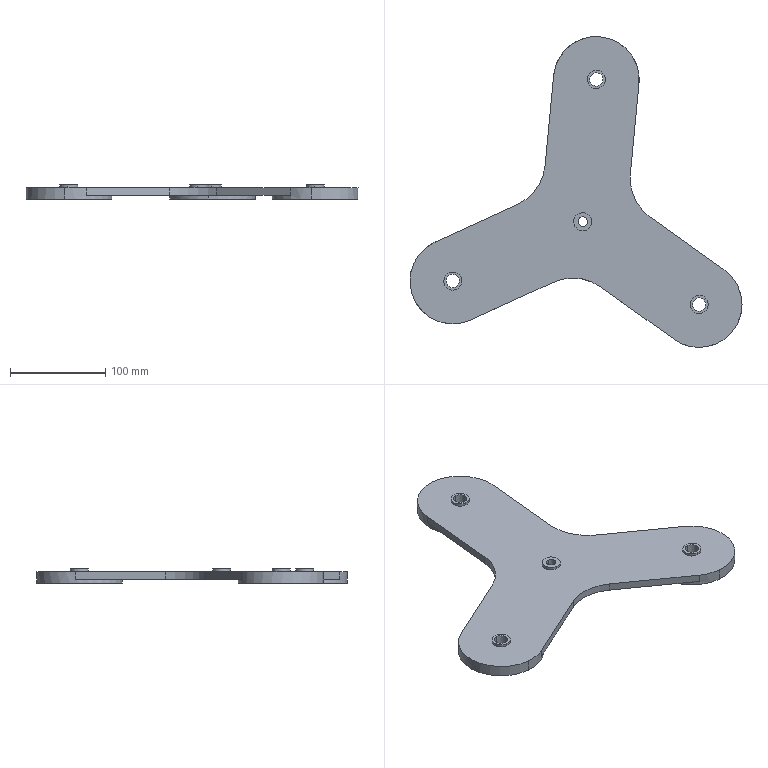Part | SolidWorks | features BaseBody 1 | 1 solid | 40 faces | box 348.636 x 326.309 x 15 mm | volume 447458 mm3 | cylinder 25 | plane 15 | commonest cylinder face diameters 19 x8 14 x6 90 x6 100 x3 10 x2
STEP:
#1=CARTESIAN_POINT('',(358.485,52.161,-468.));
#2=VERTEX_POINT('',#1);
#3=CARTESIAN_POINT('',(359.433,62.116,-468.));
#4=VERTEX_POINT('',#3);
#5=CARTESIAN_POINT('',(358.959,57.138,-468.));
#6=DIRECTION('',(0.,0.,-1.));
#7=DIRECTION('',(0.09487,0.9955,0.));
#8=AXIS2_PLACEMENT_3D('',#5,#6,#7);
#9=CIRCLE('',#8,5.);
#10=EDGE_CURVE('',#2,#4,#9,.T.);
#11=ORIENTED_EDGE('',*,*,#10,.T.);
#12=CARTESIAN_POINT('',(359.433,62.116,-457.));
#13=VERTEX_POINT('',#12);
#14=CARTESIAN_POINT('',(359.433,62.116,-472.));
#15=DIRECTION('',(0.,0.,1.));
#16=VECTOR('',#15,1000.);
#17=LINE('',#14,#16);
#18=EDGE_CURVE('',#4,#13,#17,.T.);
#19=ORIENTED_EDGE('',*,*,#18,.T.);
#20=CARTESIAN_POINT('',(358.485,52.161,-457.));
#21=VERTEX_POINT('',#20);
#22=CARTESIAN_POINT('',(358.959,57.138,-457.));
#23=DIRECTION('',(0.,0.,1.));
#24=DIRECTION('',(-0.09487,-0.9955,0.));
#25=AXIS2_PLACEMENT_3D('',#22,#23,#24);
#26=CIRCLE('',#25,5.);
#27=EDGE_CURVE('',#13,#21,#26,.T.);
#28=ORIENTED_EDGE('',*,*,#27,.T.);
#29=CARTESIAN_POINT('',(358.485,52.161,-472.));
#30=DIRECTION('',(0.,0.,1.));
#31=VECTOR('',#30,1000.);
#32=LINE('',#29,#31);
#33=EDGE_CURVE('',#2,#21,#32,.T.);
#34=ORIENTED_EDGE('',*,*,#33,.F.);
#35=EDGE_LOOP('',(#11,#19,#28,#34));
#36=FACE_OUTER_BOUND('',#35,.T.);
#37=CARTESIAN_POINT('',(358.959,57.138,-472.));
#38=DIRECTION('',(0.,0.,1.));
#39=DIRECTION('',(-0.09487,-0.9955,0.));
#40=AXIS2_PLACEMENT_3D('',#37,#38,#39);
#41=CYLINDRICAL_SURFACE('',#40,5.);
#42=ADVANCED_FACE('',(#36),#41,.F.);
#43=CARTESIAN_POINT('',(373.853,213.43,-472.));
#44=VERTEX_POINT('',#43);
#45=CARTESIAN_POINT('',(372.525,199.493,-472.));
#46=VERTEX_POINT('',#45);
#47=CARTESIAN_POINT('',(373.189,206.462,-472.));
#48=DIRECTION('',(0.,0.,1.));
#49=DIRECTION('',(-0.09487,-0.9955,0.));
#50=AXIS2_PLACEMENT_3D('',#47,#48,#49);
#51=CIRCLE('',#50,7.);
#52=EDGE_CURVE('',#44,#46,#51,.T.);
#53=ORIENTED_EDGE('',*,*,#52,.F.);
#54=CARTESIAN_POINT('',(373.853,213.43,-457.));
#55=VERTEX_POINT('',#54);
#56=CARTESIAN_POINT('',(373.853,213.43,-472.));
#57=DIRECTION('',(0.,0.,1.));
#58=VECTOR('',#57,1000.);
#59=LINE('',#56,#58);
#60=EDGE_CURVE('',#44,#55,#59,.T.);
#61=ORIENTED_EDGE('',*,*,#60,.T.);
#62=CARTESIAN_POINT('',(372.525,199.493,-457.));
#63=VERTEX_POINT('',#62);
#64=CARTESIAN_POINT('',(373.189,206.462,-457.));
#65=DIRECTION('',(0.,0.,1.));
#66=DIRECTION('',(-0.09487,-0.9955,0.));
#67=AXIS2_PLACEMENT_3D('',#64,#65,#66);
#68=CIRCLE('',#67,7.);
#69=EDGE_CURVE('',#55,#63,#68,.T.);
#70=ORIENTED_EDGE('',*,*,#69,.T.);
#71=CARTESIAN_POINT('',(372.525,199.493,-472.));
#72=DIRECTION('',(0.,0.,1.));
#73=VECTOR('',#72,1000.);
#74=LINE('',#71,#73);
#75=EDGE_CURVE('',#46,#63,#74,.T.);
#76=ORIENTED_EDGE('',*,*,#75,.F.);
#77=EDGE_LOOP('',(#53,#61,#70,#76));
#78=FACE_OUTER_BOUND('',#77,.T.);
#79=CARTESIAN_POINT('',(373.189,206.462,-472.));
#80=DIRECTION('',(0.,0.,1.));
#81=DIRECTION('',(-0.09487,-0.9955,0.));
#82=AXIS2_PLACEMENT_3D('',#79,#80,#81);
#83=CYLINDRICAL_SURFACE('',#82,7.);
#84=ADVANCED_FACE('',(#78),#83,.F.);
#85=CARTESIAN_POINT('',(223.19,1.768,-472.));
#86=VERTEX_POINT('',#85);
#87=CARTESIAN_POINT('',(221.862,-12.168,-472.));
#88=VERTEX_POINT('',#87);
#89=CARTESIAN_POINT('',(222.526,-5.2,-472.));
#90=DIRECTION('',(0.,0.,1.));
#91=DIRECTION('',(-0.09487,-0.9955,0.));
#92=AXIS2_PLACEMENT_3D('',#89,#90,#91);
#93=CIRCLE('',#92,7.);
#94=EDGE_CURVE('',#86,#88,#93,.T.);
#95=ORIENTED_EDGE('',*,*,#94,.F.);
#96=CARTESIAN_POINT('',(223.19,1.768,-457.));
#97=VERTEX_POINT('',#96);
#98=CARTESIAN_POINT('',(223.19,1.768,-472.));
#99=DIRECTION('',(0.,0.,1.));
#100=VECTOR('',#99,1000.);
#101=LINE('',#98,#100);
#102=EDGE_CURVE('',#86,#97,#101,.T.);
#103=ORIENTED_EDGE('',*,*,#102,.T.);
#104=CARTESIAN_POINT('',(221.862,-12.168,-457.));
#105=VERTEX_POINT('',#104);
#106=CARTESIAN_POINT('',(222.526,-5.2,-457.));
#107=DIRECTION('',(0.,0.,1.));
#108=DIRECTION('',(-0.09487,-0.9955,0.));
#109=AXIS2_PLACEMENT_3D('',#106,#107,#108);
#110=CIRCLE('',#109,7.);
#111=EDGE_CURVE('',#97,#105,#110,.T.);
#112=ORIENTED_EDGE('',*,*,#111,.T.);
#113=CARTESIAN_POINT('',(221.862,-12.168,-472.));
#114=DIRECTION('',(0.,0.,1.));
#115=VECTOR('',#114,1000.);
#116=LINE('',#113,#115);
#117=EDGE_CURVE('',#88,#105,#116,.T.);
#118=ORIENTED_EDGE('',*,*,#117,.F.);
#119=EDGE_LOOP('',(#95,#103,#112,#118));
#120=FACE_OUTER_BOUND('',#119,.T.);
#121=CARTESIAN_POINT('',(222.526,-5.2,-472.));
#122=DIRECTION('',(0.,0.,1.));
#123=DIRECTION('',(-0.09487,-0.9955,0.));
#124=AXIS2_PLACEMENT_3D('',#121,#122,#123);
#125=CYLINDRICAL_SURFACE('',#124,7.);
#126=ADVANCED_FACE('',(#120),#125,.F.);
#127=CARTESIAN_POINT('',(481.826,-22.878,-472.));
#128=VERTEX_POINT('',#127);
#129=CARTESIAN_POINT('',(480.498,-36.815,-472.));
#130=VERTEX_POINT('',#129);
#131=CARTESIAN_POINT('',(481.162,-29.847,-472.));
#132=DIRECTION('',(0.,0.,1.));
#133=DIRECTION('',(-0.09487,-0.9955,0.));
#134=AXIS2_PLACEMENT_3D('',#131,#132,#133);
#135=CIRCLE('',#134,7.);
#136=EDGE_CURVE('',#128,#130,#135,.T.);
#137=ORIENTED_EDGE('',*,*,#136,.F.);
#138=CARTESIAN_POINT('',(481.826,-22.878,-457.));
#139=VERTEX_POINT('',#138);
#140=CARTESIAN_POINT('',(481.826,-22.878,-472.));
#141=DIRECTION('',(0.,0.,1.));
#142=VECTOR('',#141,1000.);
#143=LINE('',#140,#142);
#144=EDGE_CURVE('',#128,#139,#143,.T.);
#145=ORIENTED_EDGE('',*,*,#144,.T.);
#146=CARTESIAN_POINT('',(480.498,-36.815,-457.));
#147=VERTEX_POINT('',#146);
#148=CARTESIAN_POINT('',(481.162,-29.847,-457.));
#149=DIRECTION('',(0.,0.,1.));
#150=DIRECTION('',(-0.09487,-0.9955,0.));
#151=AXIS2_PLACEMENT_3D('',#148,#149,#150);
#152=CIRCLE('',#151,7.);
#153=EDGE_CURVE('',#139,#147,#152,.T.);
#154=ORIENTED_EDGE('',*,*,#153,.T.);
#155=CARTESIAN_POINT('',(480.498,-36.815,-472.));
#156=DIRECTION('',(0.,0.,1.));
#157=VECTOR('',#156,1000.);
#158=LINE('',#155,#157);
#159=EDGE_CURVE('',#130,#147,#158,.T.);
#160=ORIENTED_EDGE('',*,*,#159,.F.);
#161=EDGE_LOOP('',(#137,#145,#154,#160));
#162=FACE_OUTER_BOUND('',#161,.T.);
#163=CARTESIAN_POINT('',(481.162,-29.847,-472.));
#164=DIRECTION('',(0.,0.,1.));
#165=DIRECTION('',(-0.09487,-0.9955,0.));
#166=AXIS2_PLACEMENT_3D('',#163,#164,#165);
#167=CYLINDRICAL_SURFACE('',#166,7.);
#168=ADVANCED_FACE('',(#162),#167,.F.);
#169=CARTESIAN_POINT('',(358.058,47.681,-457.));
#170=VERTEX_POINT('',#169);
#171=CARTESIAN_POINT('',(359.86,66.596,-457.));
#172=VERTEX_POINT('',#171);
#173=CARTESIAN_POINT('',(358.959,57.138,-457.));
#174=DIRECTION('',(0.,0.,1.));
#175=DIRECTION('',(-0.09487,-0.9955,0.));
#176=AXIS2_PLACEMENT_3D('',#173,#174,#175);
#177=CIRCLE('',#176,9.5);
#178=EDGE_CURVE('',#170,#172,#177,.T.);
#179=ORIENTED_EDGE('',*,*,#178,.F.);
#180=CARTESIAN_POINT('',(358.058,47.681,-460.));
#181=VERTEX_POINT('',#180);
#182=CARTESIAN_POINT('',(358.058,47.681,-457.));
#183=DIRECTION('',(0.,0.,-1.));
#184=VECTOR('',#183,1000.);
#185=LINE('',#182,#184);
#186=EDGE_CURVE('',#170,#181,#185,.T.);
#187=ORIENTED_EDGE('',*,*,#186,.T.);
#188=CARTESIAN_POINT('',(359.86,66.596,-460.));
#189=VERTEX_POINT('',#188);
#190=CARTESIAN_POINT('',(358.959,57.138,-460.));
#191=DIRECTION('',(0.,0.,1.));
#192=DIRECTION('',(0.09487,0.9955,0.));
#193=AXIS2_PLACEMENT_3D('',#190,#191,#192);
#194=CIRCLE('',#193,9.5);
#195=EDGE_CURVE('',#181,#189,#194,.T.);
#196=ORIENTED_EDGE('',*,*,#195,.T.);
#197=CARTESIAN_POINT('',(359.86,66.596,-457.));
#198=DIRECTION('',(0.,0.,-1.));
#199=VECTOR('',#198,1000.);
#200=LINE('',#197,#199);
#201=EDGE_CURVE('',#172,#189,#200,.T.);
#202=ORIENTED_EDGE('',*,*,#201,.F.);
#203=EDGE_LOOP('',(#179,#187,#196,#202));
#204=FACE_OUTER_BOUND('',#203,.T.);
#205=CARTESIAN_POINT('',(358.959,57.138,-457.));
#206=DIRECTION('',(0.,0.,-1.));
#207=DIRECTION('',(0.09487,0.9955,0.));
#208=AXIS2_PLACEMENT_3D('',#205,#206,#207);
#209=CYLINDRICAL_SURFACE('',#208,9.5);
#210=ADVANCED_FACE('',(#204),#209,.T.);
#211=CARTESIAN_POINT('',(480.261,-39.304,-457.));
#212=VERTEX_POINT('',#211);
#213=CARTESIAN_POINT('',(482.063,-20.39,-457.));
#214=VERTEX_POINT('',#213);
#215=CARTESIAN_POINT('',(481.162,-29.847,-457.));
#216=DIRECTION('',(0.,0.,1.));
#217=DIRECTION('',(-0.09487,-0.9955,0.));
#218=AXIS2_PLACEMENT_3D('',#215,#216,#217);
#219=CIRCLE('',#218,9.5);
#220=EDGE_CURVE('',#212,#214,#219,.T.);
#221=ORIENTED_EDGE('',*,*,#220,.F.);
#222=CARTESIAN_POINT('',(480.261,-39.304,-460.));
#223=VERTEX_POINT('',#222);
#224=CARTESIAN_POINT('',(480.261,-39.304,-457.));
#225=DIRECTION('',(0.,0.,-1.));
#226=VECTOR('',#225,1000.);
#227=LINE('',#224,#226);
#228=EDGE_CURVE('',#212,#223,#227,.T.);
#229=ORIENTED_EDGE('',*,*,#228,.T.);
#230=CARTESIAN_POINT('',(482.063,-20.39,-460.));
#231=VERTEX_POINT('',#230);
#232=CARTESIAN_POINT('',(481.162,-29.847,-460.));
#233=DIRECTION('',(0.,0.,1.));
#234=DIRECTION('',(0.09487,0.9955,0.));
#235=AXIS2_PLACEMENT_3D('',#232,#233,#234);
#236=CIRCLE('',#235,9.5);
#237=EDGE_CURVE('',#223,#231,#236,.T.);
#238=ORIENTED_EDGE('',*,*,#237,.T.);
#239=CARTESIAN_POINT('',(482.063,-20.39,-457.));
#240=DIRECTION('',(0.,0.,-1.));
#241=VECTOR('',#240,1000.);
#242=LINE('',#239,#241);
#243=EDGE_CURVE('',#214,#231,#242,.T.);
#244=ORIENTED_EDGE('',*,*,#243,.F.);
#245=EDGE_LOOP('',(#221,#229,#238,#244));
#246=FACE_OUTER_BOUND('',#245,.T.);
#247=CARTESIAN_POINT('',(481.162,-29.847,-457.));
#248=DIRECTION('',(0.,0.,-1.));
#249=DIRECTION('',(0.09487,0.9955,0.));
#250=AXIS2_PLACEMENT_3D('',#247,#248,#249);
#251=CYLINDRICAL_SURFACE('',#250,9.5);
#252=ADVANCED_FACE('',(#246),#251,.T.);
#253=CARTESIAN_POINT('',(221.625,-14.657,-457.));
#254=VERTEX_POINT('',#253);
#255=CARTESIAN_POINT('',(223.427,4.257,-457.));
#256=VERTEX_POINT('',#255);
#257=CARTESIAN_POINT('',(222.526,-5.2,-457.));
#258=DIRECTION('',(0.,0.,1.));
#259=DIRECTION('',(-0.09487,-0.9955,0.));
#260=AXIS2_PLACEMENT_3D('',#257,#258,#259);
#261=CIRCLE('',#260,9.5);
#262=EDGE_CURVE('',#254,#256,#261,.T.);
#263=ORIENTED_EDGE('',*,*,#262,.F.);
#264=CARTESIAN_POINT('',(221.625,-14.657,-460.));
#265=VERTEX_POINT('',#264);
#266=CARTESIAN_POINT('',(221.625,-14.657,-457.));
#267=DIRECTION('',(0.,0.,-1.));
#268=VECTOR('',#267,1000.);
#269=LINE('',#266,#268);
#270=EDGE_CURVE('',#254,#265,#269,.T.);
#271=ORIENTED_EDGE('',*,*,#270,.T.);
#272=CARTESIAN_POINT('',(223.427,4.257,-460.));
#273=VERTEX_POINT('',#272);
#274=CARTESIAN_POINT('',(222.526,-5.2,-460.));
#275=DIRECTION('',(0.,0.,1.));
#276=DIRECTION('',(0.09487,0.9955,0.));
#277=AXIS2_PLACEMENT_3D('',#274,#275,#276);
#278=CIRCLE('',#277,9.5);
#279=EDGE_CURVE('',#265,#273,#278,.T.);
#280=ORIENTED_EDGE('',*,*,#279,.T.);
#281=CARTESIAN_POINT('',(223.427,4.257,-457.));
#282=DIRECTION('',(0.,0.,-1.));
#283=VECTOR('',#282,1000.);
#284=LINE('',#281,#283);
#285=EDGE_CURVE('',#256,#273,#284,.T.);
#286=ORIENTED_EDGE('',*,*,#285,.F.);
#287=EDGE_LOOP('',(#263,#271,#280,#286));
#288=FACE_OUTER_BOUND('',#287,.T.);
#289=CARTESIAN_POINT('',(222.526,-5.2,-457.));
#290=DIRECTION('',(0.,0.,-1.));
#291=DIRECTION('',(0.09487,0.9955,0.));
#292=AXIS2_PLACEMENT_3D('',#289,#290,#291);
#293=CYLINDRICAL_SURFACE('',#292,9.5);
#294=ADVANCED_FACE('',(#288),#293,.T.);
#295=CARTESIAN_POINT('',(372.288,197.005,-457.));
#296=VERTEX_POINT('',#295);
#297=CARTESIAN_POINT('',(374.09,215.919,-457.));
#298=VERTEX_POINT('',#297);
#299=CARTESIAN_POINT('',(373.189,206.462,-457.));
#300=DIRECTION('',(0.,0.,1.));
#301=DIRECTION('',(-0.09487,-0.9955,0.));
#302=AXIS2_PLACEMENT_3D('',#299,#300,#301);
#303=CIRCLE('',#302,9.5);
#304=EDGE_CURVE('',#296,#298,#303,.T.);
#305=ORIENTED_EDGE('',*,*,#304,.F.);
#306=CARTESIAN_POINT('',(372.288,197.005,-460.));
#307=VERTEX_POINT('',#306);
#308=CARTESIAN_POINT('',(372.288,197.005,-457.));
#309=DIRECTION('',(0.,0.,-1.));
#310=VECTOR('',#309,1000.);
#311=LINE('',#308,#310);
#312=EDGE_CURVE('',#296,#307,#311,.T.);
#313=ORIENTED_EDGE('',*,*,#312,.T.);
#314=CARTESIAN_POINT('',(374.09,215.919,-460.));
#315=VERTEX_POINT('',#314);
#316=CARTESIAN_POINT('',(373.189,206.462,-460.));
#317=DIRECTION('',(0.,0.,1.));
#318=DIRECTION('',(0.09487,0.9955,0.));
#319=AXIS2_PLACEMENT_3D('',#316,#317,#318);
#320=CIRCLE('',#319,9.5);
#321=EDGE_CURVE('',#307,#315,#320,.T.);
#322=ORIENTED_EDGE('',*,*,#321,.T.);
#323=CARTESIAN_POINT('',(374.09,215.919,-457.));
#324=DIRECTION('',(0.,0.,-1.));
#325=VECTOR('',#324,1000.);
#326=LINE('',#323,#325);
#327=EDGE_CURVE('',#298,#315,#326,.T.);
#328=ORIENTED_EDGE('',*,*,#327,.F.);
#329=EDGE_LOOP('',(#305,#313,#322,#328));
#330=FACE_OUTER_BOUND('',#329,.T.);
#331=CARTESIAN_POINT('',(373.189,206.462,-457.));
#332=DIRECTION('',(0.,0.,-1.));
#333=DIRECTION('',(0.09487,0.9955,0.));
#334=AXIS2_PLACEMENT_3D('',#331,#332,#333);
#335=CYLINDRICAL_SURFACE('',#334,9.5);
#336=ADVANCED_FACE('',(#330),#335,.T.);
#337=CARTESIAN_POINT('',(226.795,39.597,-472.));
#338=VERTEX_POINT('',#337);
#339=CARTESIAN_POINT('',(218.257,-49.997,-472.));
#340=VERTEX_POINT('',#339);
#341=CARTESIAN_POINT('',(222.526,-5.2,-472.));
#342=DIRECTION('',(0.,0.,-1.));
#343=DIRECTION('',(0.09487,0.9955,0.));
#344=AXIS2_PLACEMENT_3D('',#341,#342,#343);
#345=CIRCLE('',#344,45.);
#346=EDGE_CURVE('',#338,#340,#345,.T.);
#347=ORIENTED_EDGE('',*,*,#346,.F.);
#348=CARTESIAN_POINT('',(226.795,39.597,-468.));
#349=VERTEX_POINT('',#348);
#350=CARTESIAN_POINT('',(226.795,39.597,-468.));
#351=DIRECTION('',(0.,0.,1.));
#352=VECTOR('',#351,1000.);
#353=LINE('',#350,#352);
#354=EDGE_CURVE('',#338,#349,#353,.T.);
#355=ORIENTED_EDGE('',*,*,#354,.T.);
#356=CARTESIAN_POINT('',(241.228,-46.13,-468.));
#357=VERTEX_POINT('',#356);
#358=CARTESIAN_POINT('',(222.526,-5.2,-468.));
#359=DIRECTION('',(0.,0.,-1.));
#360=DIRECTION('',(0.09487,0.9955,0.));
#361=AXIS2_PLACEMENT_3D('',#358,#359,#360);
#362=CIRCLE('',#361,45.);
#363=EDGE_CURVE('',#349,#357,#362,.T.);
#364=ORIENTED_EDGE('',*,*,#363,.T.);
#365=CARTESIAN_POINT('',(241.228,-46.13,-460.));
#366=VERTEX_POINT('',#365);
#367=CARTESIAN_POINT('',(241.228,-46.13,-468.));
#368=DIRECTION('',(0.,0.,1.));
#369=VECTOR('',#368,1000.);
#370=LINE('',#367,#369);
#371=EDGE_CURVE('',#357,#366,#370,.T.);
#372=ORIENTED_EDGE('',*,*,#371,.T.);
#373=CARTESIAN_POINT('',(218.257,-49.997,-460.));
#374=VERTEX_POINT('',#373);
#375=CARTESIAN_POINT('',(222.526,-5.2,-460.));
#376=DIRECTION('',(0.,0.,-1.));
#377=DIRECTION('',(0.09487,0.9955,0.));
#378=AXIS2_PLACEMENT_3D('',#375,#376,#377);
#379=CIRCLE('',#378,45.);
#380=EDGE_CURVE('',#366,#374,#379,.T.);
#381=ORIENTED_EDGE('',*,*,#380,.T.);
#382=CARTESIAN_POINT('',(218.257,-49.997,-468.));
#383=DIRECTION('',(0.,0.,1.));
#384=VECTOR('',#383,1000.);
#385=LINE('',#382,#384);
#386=EDGE_CURVE('',#340,#374,#385,.T.);
#387=ORIENTED_EDGE('',*,*,#386,.F.);
#388=EDGE_LOOP('',(#347,#355,#364,#372,#381,#387));
#389=FACE_OUTER_BOUND('',#388,.T.);
#390=CARTESIAN_POINT('',(222.526,-5.2,-468.));
#391=DIRECTION('',(0.,0.,1.));
#392=DIRECTION('',(-0.09487,-0.9955,0.));
#393=AXIS2_PLACEMENT_3D('',#390,#391,#392);
#394=CYLINDRICAL_SURFACE('',#393,45.);
#395=ADVANCED_FACE('',(#389),#394,.T.);
#396=CARTESIAN_POINT('',(485.431,14.95,-472.));
#397=VERTEX_POINT('',#396);
#398=CARTESIAN_POINT('',(476.893,-74.644,-472.));
#399=VERTEX_POINT('',#398);
#400=CARTESIAN_POINT('',(481.162,-29.847,-472.));
#401=DIRECTION('',(0.,0.,-1.));
#402=DIRECTION('',(0.09487,0.9955,0.));
#403=AXIS2_PLACEMENT_3D('',#400,#401,#402);
#404=CIRCLE('',#403,45.);
#405=EDGE_CURVE('',#397,#399,#404,.T.);
#406=ORIENTED_EDGE('',*,*,#405,.F.);
#407=CARTESIAN_POINT('',(485.431,14.95,-468.));
#408=VERTEX_POINT('',#407);
#409=CARTESIAN_POINT('',(485.431,14.95,-468.));
#410=DIRECTION('',(0.,0.,1.));
#411=VECTOR('',#410,1000.);
#412=LINE('',#409,#411);
#413=EDGE_CURVE('',#397,#408,#412,.T.);
#414=ORIENTED_EDGE('',*,*,#413,.T.);
#415=CARTESIAN_POINT('',(507.258,6.814,-468.));
#416=VERTEX_POINT('',#415);
#417=CARTESIAN_POINT('',(481.162,-29.847,-468.));
#418=DIRECTION('',(0.,0.,-1.));
#419=DIRECTION('',(0.09487,0.9955,0.));
#420=AXIS2_PLACEMENT_3D('',#417,#418,#419);
#421=CIRCLE('',#420,45.);
#422=EDGE_CURVE('',#408,#416,#421,.T.);
#423=ORIENTED_EDGE('',*,*,#422,.T.);
#424=CARTESIAN_POINT('',(507.258,6.814,-460.));
#425=VERTEX_POINT('',#424);
#426=CARTESIAN_POINT('',(507.258,6.814,-468.));
#427=DIRECTION('',(0.,0.,1.));
#428=VECTOR('',#427,1000.);
#429=LINE('',#426,#428);
#430=EDGE_CURVE('',#416,#425,#429,.T.);
#431=ORIENTED_EDGE('',*,*,#430,.T.);
#432=CARTESIAN_POINT('',(476.893,-74.644,-460.));
#433=VERTEX_POINT('',#432);
#434=CARTESIAN_POINT('',(481.162,-29.847,-460.));
#435=DIRECTION('',(0.,0.,-1.));
#436=DIRECTION('',(0.09487,0.9955,0.));
#437=AXIS2_PLACEMENT_3D('',#434,#435,#436);
#438=CIRCLE('',#437,45.);
#439=EDGE_CURVE('',#425,#433,#438,.T.);
#440=ORIENTED_EDGE('',*,*,#439,.T.);
#441=CARTESIAN_POINT('',(476.893,-74.644,-468.));
#442=DIRECTION('',(0.,0.,1.));
#443=VECTOR('',#442,1000.);
#444=LINE('',#441,#443);
#445=EDGE_CURVE('',#399,#433,#444,.T.);
#446=ORIENTED_EDGE('',*,*,#445,.F.);
#447=EDGE_LOOP('',(#406,#414,#423,#431,#440,#446));
#448=FACE_OUTER_BOUND('',#447,.T.);
#449=CARTESIAN_POINT('',(481.162,-29.847,-468.));
#450=DIRECTION('',(0.,0.,1.));
#451=DIRECTION('',(-0.09487,-0.9955,0.));
#452=AXIS2_PLACEMENT_3D('',#449,#450,#451);
#453=CYLINDRICAL_SURFACE('',#452,45.);
#454=ADVANCED_FACE('',(#448),#453,.T.);
#455=CARTESIAN_POINT('',(377.458,251.259,-472.));
#456=VERTEX_POINT('',#455);
#457=CARTESIAN_POINT('',(368.92,161.665,-472.));
#458=VERTEX_POINT('',#457);
#459=CARTESIAN_POINT('',(373.189,206.462,-472.));
#460=DIRECTION('',(0.,0.,-1.));
#461=DIRECTION('',(0.09487,0.9955,0.));
#462=AXIS2_PLACEMENT_3D('',#459,#460,#461);
#463=CIRCLE('',#462,45.);
#464=EDGE_CURVE('',#456,#458,#463,.T.);
#465=ORIENTED_EDGE('',*,*,#464,.F.);
#466=CARTESIAN_POINT('',(377.458,251.259,-460.));
#467=VERTEX_POINT('',#466);
#468=CARTESIAN_POINT('',(377.458,251.259,-468.));
#469=DIRECTION('',(0.,0.,1.));
#470=VECTOR('',#469,1000.);
#471=LINE('',#468,#470);
#472=EDGE_CURVE('',#456,#467,#471,.T.);
#473=ORIENTED_EDGE('',*,*,#472,.T.);
#474=CARTESIAN_POINT('',(417.986,202.193,-460.));
#475=VERTEX_POINT('',#474);
#476=CARTESIAN_POINT('',(373.189,206.462,-460.));
#477=DIRECTION('',(0.,0.,-1.));
#478=DIRECTION('',(0.09487,0.9955,0.));
#479=AXIS2_PLACEMENT_3D('',#476,#477,#478);
#480=CIRCLE('',#479,45.);
#481=EDGE_CURVE('',#467,#475,#480,.T.);
#482=ORIENTED_EDGE('',*,*,#481,.T.);
#483=CARTESIAN_POINT('',(417.986,202.193,-468.));
#484=VERTEX_POINT('',#483);
#485=CARTESIAN_POINT('',(417.986,202.193,-468.));
#486=DIRECTION('',(0.,0.,1.));
#487=VECTOR('',#486,1000.);
#488=LINE('',#485,#487);
#489=EDGE_CURVE('',#484,#475,#488,.T.);
#490=ORIENTED_EDGE('',*,*,#489,.F.);
#491=CARTESIAN_POINT('',(368.92,161.665,-468.));
#492=VERTEX_POINT('',#491);
#493=CARTESIAN_POINT('',(373.189,206.462,-468.));
#494=DIRECTION('',(0.,0.,-1.));
#495=DIRECTION('',(0.09487,0.9955,0.));
#496=AXIS2_PLACEMENT_3D('',#493,#494,#495);
#497=CIRCLE('',#496,45.);
#498=EDGE_CURVE('',#484,#492,#497,.T.);
#499=ORIENTED_EDGE('',*,*,#498,.T.);
#500=CARTESIAN_POINT('',(368.92,161.665,-468.));
#501=DIRECTION('',(0.,0.,1.));
#502=VECTOR('',#501,1000.);
#503=LINE('',#500,#502);
#504=EDGE_CURVE('',#458,#492,#503,.T.);
#505=ORIENTED_EDGE('',*,*,#504,.F.);
#506=EDGE_LOOP('',(#465,#473,#482,#490,#499,#505));
#507=FACE_OUTER_BOUND('',#506,.T.);
#508=CARTESIAN_POINT('',(373.189,206.462,-468.));
#509=DIRECTION('',(0.,0.,1.));
#510=DIRECTION('',(-0.09487,-0.9955,0.));
#511=AXIS2_PLACEMENT_3D('',#508,#509,#510);
#512=CYLINDRICAL_SURFACE('',#511,45.);
#513=ADVANCED_FACE('',(#507),#512,.T.);
#514=CARTESIAN_POINT('',(481.162,-29.847,-460.));
#515=DIRECTION('',(0.,0.,1.));
#516=DIRECTION('',(0.09487,0.9955,0.));
#517=AXIS2_PLACEMENT_3D('',#514,#515,#516);
#518=CIRCLE('',#517,9.5);
#519=EDGE_CURVE('',#231,#223,#518,.T.);
#520=ORIENTED_EDGE('',*,*,#519,.F.);
#521=ORIENTED_EDGE('',*,*,#237,.F.);
#522=EDGE_LOOP('',(#520,#521));
#523=FACE_BOUND('',#522,.T.);
#524=CARTESIAN_POINT('',(373.189,206.462,-460.));
#525=DIRECTION('',(0.,0.,1.));
#526=DIRECTION('',(0.09487,0.9955,0.));
#527=AXIS2_PLACEMENT_3D('',#524,#525,#526);
#528=CIRCLE('',#527,9.5);
#529=EDGE_CURVE('',#315,#307,#528,.T.);
#530=ORIENTED_EDGE('',*,*,#529,.F.);
#531=ORIENTED_EDGE('',*,*,#321,.F.);
#532=EDGE_LOOP('',(#530,#531));
#533=FACE_BOUND('',#532,.T.);
#534=CARTESIAN_POINT('',(328.392,210.731,-460.));
#535=VERTEX_POINT('',#534);
#536=CARTESIAN_POINT('',(373.189,206.462,-460.));
#537=DIRECTION('',(0.,0.,-1.));
#538=DIRECTION('',(0.09487,0.9955,0.));
#539=AXIS2_PLACEMENT_3D('',#536,#537,#538);
#540=CIRCLE('',#539,45.);
#541=EDGE_CURVE('',#535,#467,#540,.T.);
#542=ORIENTED_EDGE('',*,*,#541,.F.);
#543=CARTESIAN_POINT('',(319.365,116.008,-460.));
#544=VERTEX_POINT('',#543);
#545=CARTESIAN_POINT('',(328.392,210.731,-460.));
#546=DIRECTION('',(0.09487,0.9955,0.));
#547=VECTOR('',#546,1000.);
#548=LINE('',#545,#547);
#549=EDGE_CURVE('',#544,#535,#548,.T.);
#550=ORIENTED_EDGE('',*,*,#549,.F.);
#551=CARTESIAN_POINT('',(290.37,75.274,-460.));
#552=VERTEX_POINT('',#551);
#553=CARTESIAN_POINT('',(269.591,120.752,-460.));
#554=DIRECTION('',(0.,0.,1.));
#555=DIRECTION('',(0.09487,0.9955,0.));
#556=AXIS2_PLACEMENT_3D('',#553,#554,#555);
#557=CIRCLE('',#556,50.);
#558=EDGE_CURVE('',#552,#544,#557,.T.);
#559=ORIENTED_EDGE('',*,*,#558,.F.);
#560=CARTESIAN_POINT('',(203.825,35.73,-460.));
#561=VERTEX_POINT('',#560);
#562=CARTESIAN_POINT('',(203.825,35.73,-460.));
#563=DIRECTION('',(0.9096,0.4156,0.));
#564=VECTOR('',#563,1000.);
#565=LINE('',#562,#564);
#566=EDGE_CURVE('',#561,#552,#565,.T.);
#567=ORIENTED_EDGE('',*,*,#566,.F.);
#568=CARTESIAN_POINT('',(222.526,-5.2,-460.));
#569=DIRECTION('',(0.,0.,-1.));
#570=DIRECTION('',(0.09487,0.9955,0.));
#571=AXIS2_PLACEMENT_3D('',#568,#569,#570);
#572=CIRCLE('',#571,45.);
#573=EDGE_CURVE('',#374,#561,#572,.T.);
#574=ORIENTED_EDGE('',*,*,#573,.F.);
#575=ORIENTED_EDGE('',*,*,#380,.F.);
#576=CARTESIAN_POINT('',(327.773,-6.586,-460.));
#577=VERTEX_POINT('',#576);
#578=CARTESIAN_POINT('',(241.228,-46.13,-460.));
#579=DIRECTION('',(-0.9096,-0.4156,0.));
#580=VECTOR('',#579,1000.);
#581=LINE('',#578,#580);
#582=EDGE_CURVE('',#577,#366,#581,.T.);
#583=ORIENTED_EDGE('',*,*,#582,.F.);
#584=CARTESIAN_POINT('',(377.548,-11.329,-460.));
#585=VERTEX_POINT('',#584);
#586=CARTESIAN_POINT('',(348.553,-52.063,-460.));
#587=DIRECTION('',(0.,0.,1.));
#588=DIRECTION('',(-0.09487,-0.9955,0.));
#589=AXIS2_PLACEMENT_3D('',#586,#587,#588);
#590=CIRCLE('',#589,50.);
#591=EDGE_CURVE('',#585,#577,#590,.T.);
#592=ORIENTED_EDGE('',*,*,#591,.F.);
#593=CARTESIAN_POINT('',(455.067,-66.508,-460.));
#594=VERTEX_POINT('',#593);
#595=CARTESIAN_POINT('',(455.067,-66.508,-460.));
#596=DIRECTION('',(-0.8147,0.5799,0.));
#597=VECTOR('',#596,1000.);
#598=LINE('',#595,#597);
#599=EDGE_CURVE('',#594,#585,#598,.T.);
#600=ORIENTED_EDGE('',*,*,#599,.F.);
#601=CARTESIAN_POINT('',(481.162,-29.847,-460.));
#602=DIRECTION('',(0.,0.,-1.));
#603=DIRECTION('',(0.09487,0.9955,0.));
#604=AXIS2_PLACEMENT_3D('',#601,#602,#603);
#605=CIRCLE('',#604,45.);
#606=EDGE_CURVE('',#433,#594,#605,.T.);
#607=ORIENTED_EDGE('',*,*,#606,.F.);
#608=ORIENTED_EDGE('',*,*,#439,.F.);
#609=CARTESIAN_POINT('',(429.739,61.993,-460.));
#610=VERTEX_POINT('',#609);
#611=CARTESIAN_POINT('',(507.258,6.814,-460.));
#612=DIRECTION('',(0.8147,-0.5799,0.));
#613=VECTOR('',#612,1000.);
#614=LINE('',#611,#613);
#615=EDGE_CURVE('',#610,#425,#614,.T.);
#616=ORIENTED_EDGE('',*,*,#615,.F.);
#617=CARTESIAN_POINT('',(408.959,107.47,-460.));
#618=VERTEX_POINT('',#617);
#619=CARTESIAN_POINT('',(458.734,102.727,-460.));
#620=DIRECTION('',(0.,0.,1.));
#621=DIRECTION('',(-0.09487,-0.9955,0.));
#622=AXIS2_PLACEMENT_3D('',#619,#620,#621);
#623=CIRCLE('',#622,50.);
#624=EDGE_CURVE('',#618,#610,#623,.T.);
#625=ORIENTED_EDGE('',*,*,#624,.F.);
#626=CARTESIAN_POINT('',(417.986,202.193,-460.));
#627=DIRECTION('',(-0.09487,-0.9955,0.));
#628=VECTOR('',#627,1000.);
#629=LINE('',#626,#628);
#630=EDGE_CURVE('',#475,#618,#629,.T.);
#631=ORIENTED_EDGE('',*,*,#630,.F.);
#632=ORIENTED_EDGE('',*,*,#481,.F.);
#633=EDGE_LOOP('',(#542,#550,#559,#567,#574,#575,#583,#592,#600,#607,#608,#616,#625,#631,#632));
#634=FACE_OUTER_BOUND('',#633,.T.);
#635=CARTESIAN_POINT('',(222.526,-5.2,-460.));
#636=DIRECTION('',(0.,0.,1.));
#637=DIRECTION('',(0.09487,0.9955,0.));
#638=AXIS2_PLACEMENT_3D('',#635,#636,#637);
#639=CIRCLE('',#638,9.5);
#640=EDGE_CURVE('',#273,#265,#639,.T.);
#641=ORIENTED_EDGE('',*,*,#640,.F.);
#642=ORIENTED_EDGE('',*,*,#279,.F.);
#643=EDGE_LOOP('',(#641,#642));
#644=FACE_BOUND('',#643,.T.);
#645=CARTESIAN_POINT('',(358.959,57.138,-460.));
#646=DIRECTION('',(0.,0.,1.));
#647=DIRECTION('',(0.09487,0.9955,0.));
#648=AXIS2_PLACEMENT_3D('',#645,#646,#647);
#649=CIRCLE('',#648,9.5);
#650=EDGE_CURVE('',#189,#181,#649,.T.);
#651=ORIENTED_EDGE('',*,*,#650,.F.);
#652=ORIENTED_EDGE('',*,*,#195,.F.);
#653=EDGE_LOOP('',(#651,#652));
#654=FACE_BOUND('',#653,.T.);
#655=CARTESIAN_POINT('',(373.189,206.462,-460.));
#656=DIRECTION('',(0.,0.,-1.));
#657=DIRECTION('',(0.09487,0.9955,0.));
#658=AXIS2_PLACEMENT_3D('',#655,#656,#657);
#659=PLANE('',#658);
#660=ADVANCED_FACE('',(#523,#533,#634,#644,#654),#659,.F.);
#661=ORIENTED_EDGE('',*,*,#10,.F.);
#662=CARTESIAN_POINT('',(358.959,57.138,-468.));
#663=DIRECTION('',(0.,0.,-1.));
#664=DIRECTION('',(0.09487,0.9955,0.));
#665=AXIS2_PLACEMENT_3D('',#662,#663,#664);
#666=CIRCLE('',#665,5.);
#667=EDGE_CURVE('',#4,#2,#666,.T.);
#668=ORIENTED_EDGE('',*,*,#667,.F.);
#669=EDGE_LOOP('',(#661,#668));
#670=FACE_BOUND('',#669,.T.);
#671=CARTESIAN_POINT('',(327.773,-6.586,-468.));
#672=VERTEX_POINT('',#671);
#673=CARTESIAN_POINT('',(241.228,-46.13,-468.));
#674=DIRECTION('',(-0.9096,-0.4156,0.));
#675=VECTOR('',#674,1000.);
#676=LINE('',#673,#675);
#677=EDGE_CURVE('',#672,#357,#676,.T.);
#678=ORIENTED_EDGE('',*,*,#677,.T.);
#679=ORIENTED_EDGE('',*,*,#363,.F.);
#680=CARTESIAN_POINT('',(203.825,35.73,-468.));
#681=VERTEX_POINT('',#680);
#682=CARTESIAN_POINT('',(222.526,-5.2,-468.));
#683=DIRECTION('',(0.,0.,-1.));
#684=DIRECTION('',(0.09487,0.9955,0.));
#685=AXIS2_PLACEMENT_3D('',#682,#683,#684);
#686=CIRCLE('',#685,45.);
#687=EDGE_CURVE('',#681,#349,#686,.T.);
#688=ORIENTED_EDGE('',*,*,#687,.F.);
#689=CARTESIAN_POINT('',(290.37,75.274,-468.));
#690=VERTEX_POINT('',#689);
#691=CARTESIAN_POINT('',(203.825,35.73,-468.));
#692=DIRECTION('',(0.9096,0.4156,0.));
#693=VECTOR('',#692,1000.);
#694=LINE('',#691,#693);
#695=EDGE_CURVE('',#681,#690,#694,.T.);
#696=ORIENTED_EDGE('',*,*,#695,.T.);
#697=CARTESIAN_POINT('',(319.365,116.008,-468.));
#698=VERTEX_POINT('',#697);
#699=CARTESIAN_POINT('',(269.591,120.752,-468.));
#700=DIRECTION('',(0.,0.,1.));
#701=DIRECTION('',(0.09487,0.9955,0.));
#702=AXIS2_PLACEMENT_3D('',#699,#700,#701);
#703=CIRCLE('',#702,50.);
#704=EDGE_CURVE('',#690,#698,#703,.T.);
#705=ORIENTED_EDGE('',*,*,#704,.T.);
#706=CARTESIAN_POINT('',(328.392,210.731,-468.));
#707=VERTEX_POINT('',#706);
#708=CARTESIAN_POINT('',(328.392,210.731,-468.));
#709=DIRECTION('',(0.09487,0.9955,0.));
#710=VECTOR('',#709,1000.);
#711=LINE('',#708,#710);
#712=EDGE_CURVE('',#698,#707,#711,.T.);
#713=ORIENTED_EDGE('',*,*,#712,.T.);
#714=CARTESIAN_POINT('',(373.189,206.462,-468.));
#715=DIRECTION('',(0.,0.,-1.));
#716=DIRECTION('',(0.09487,0.9955,0.));
#717=AXIS2_PLACEMENT_3D('',#714,#715,#716);
#718=CIRCLE('',#717,45.);
#719=EDGE_CURVE('',#492,#707,#718,.T.);
#720=ORIENTED_EDGE('',*,*,#719,.F.);
#721=ORIENTED_EDGE('',*,*,#498,.F.);
#722=CARTESIAN_POINT('',(408.959,107.47,-468.));
#723=VERTEX_POINT('',#722);
#724=CARTESIAN_POINT('',(417.986,202.193,-468.));
#725=DIRECTION('',(-0.09487,-0.9955,0.));
#726=VECTOR('',#725,1000.);
#727=LINE('',#724,#726);
#728=EDGE_CURVE('',#484,#723,#727,.T.);
#729=ORIENTED_EDGE('',*,*,#728,.T.);
#730=CARTESIAN_POINT('',(429.739,61.993,-468.));
#731=VERTEX_POINT('',#730);
#732=CARTESIAN_POINT('',(458.734,102.727,-468.));
#733=DIRECTION('',(0.,0.,1.));
#734=DIRECTION('',(-0.09487,-0.9955,0.));
#735=AXIS2_PLACEMENT_3D('',#732,#733,#734);
#736=CIRCLE('',#735,50.);
#737=EDGE_CURVE('',#723,#731,#736,.T.);
#738=ORIENTED_EDGE('',*,*,#737,.T.);
#739=CARTESIAN_POINT('',(507.258,6.814,-468.));
#740=DIRECTION('',(0.8147,-0.5799,0.));
#741=VECTOR('',#740,1000.);
#742=LINE('',#739,#741);
#743=EDGE_CURVE('',#731,#416,#742,.T.);
#744=ORIENTED_EDGE('',*,*,#743,.T.);
#745=ORIENTED_EDGE('',*,*,#422,.F.);
#746=CARTESIAN_POINT('',(455.067,-66.508,-468.));
#747=VERTEX_POINT('',#746);
#748=CARTESIAN_POINT('',(481.162,-29.847,-468.));
#749=DIRECTION('',(0.,0.,-1.));
#750=DIRECTION('',(0.09487,0.9955,0.));
#751=AXIS2_PLACEMENT_3D('',#748,#749,#750);
#752=CIRCLE('',#751,45.);
#753=EDGE_CURVE('',#747,#408,#752,.T.);
#754=ORIENTED_EDGE('',*,*,#753,.F.);
#755=CARTESIAN_POINT('',(377.548,-11.329,-468.));
#756=VERTEX_POINT('',#755);
#757=CARTESIAN_POINT('',(455.067,-66.508,-468.));
#758=DIRECTION('',(-0.8147,0.5799,0.));
#759=VECTOR('',#758,1000.);
#760=LINE('',#757,#759);
#761=EDGE_CURVE('',#747,#756,#760,.T.);
#762=ORIENTED_EDGE('',*,*,#761,.T.);
#763=CARTESIAN_POINT('',(348.553,-52.063,-468.));
#764=DIRECTION('',(0.,0.,1.));
#765=DIRECTION('',(-0.09487,-0.9955,0.));
#766=AXIS2_PLACEMENT_3D('',#763,#764,#765);
#767=CIRCLE('',#766,50.);
#768=EDGE_CURVE('',#756,#672,#767,.T.);
#769=ORIENTED_EDGE('',*,*,#768,.T.);
#770=EDGE_LOOP('',(#678,#679,#688,#696,#705,#713,#720,#721,#729,#738,#744,#745,#754,#762,#769));
#771=FACE_OUTER_BOUND('',#770,.T.);
#772=CARTESIAN_POINT('',(373.189,206.462,-468.));
#773=DIRECTION('',(0.,0.,-1.));
#774=DIRECTION('',(0.09487,0.9955,0.));
#775=AXIS2_PLACEMENT_3D('',#772,#773,#774);
#776=PLANE('',#775);
#777=ADVANCED_FACE('',(#670,#771),#776,.T.);
#778=ORIENTED_EDGE('',*,*,#472,.F.);
#779=CARTESIAN_POINT('',(373.189,206.462,-472.));
#780=DIRECTION('',(0.,0.,-1.));
#781=DIRECTION('',(0.09487,0.9955,0.));
#782=AXIS2_PLACEMENT_3D('',#779,#780,#781);
#783=CIRCLE('',#782,45.);
#784=EDGE_CURVE('',#458,#456,#783,.T.);
#785=ORIENTED_EDGE('',*,*,#784,.F.);
#786=ORIENTED_EDGE('',*,*,#504,.T.);
#787=ORIENTED_EDGE('',*,*,#719,.T.);
#788=CARTESIAN_POINT('',(328.392,210.731,-468.));
#789=DIRECTION('',(0.,0.,1.));
#790=VECTOR('',#789,1000.);
#791=LINE('',#788,#790);
#792=EDGE_CURVE('',#707,#535,#791,.T.);
#793=ORIENTED_EDGE('',*,*,#792,.T.);
#794=ORIENTED_EDGE('',*,*,#541,.T.);
#795=EDGE_LOOP('',(#778,#785,#786,#787,#793,#794));
#796=FACE_OUTER_BOUND('',#795,.T.);
#797=CARTESIAN_POINT('',(373.189,206.462,-468.));
#798=DIRECTION('',(0.,0.,1.));
#799=DIRECTION('',(-0.09487,-0.9955,0.));
#800=AXIS2_PLACEMENT_3D('',#797,#798,#799);
#801=CYLINDRICAL_SURFACE('',#800,45.);
#802=ADVANCED_FACE('',(#796),#801,.T.);
#803=ORIENTED_EDGE('',*,*,#630,.T.);
#804=CARTESIAN_POINT('',(408.959,107.47,-468.));
#805=DIRECTION('',(0.,0.,1.));
#806=VECTOR('',#805,1000.);
#807=LINE('',#804,#806);
#808=EDGE_CURVE('',#723,#618,#807,.T.);
#809=ORIENTED_EDGE('',*,*,#808,.F.);
#810=ORIENTED_EDGE('',*,*,#728,.F.);
#811=ORIENTED_EDGE('',*,*,#489,.T.);
#812=EDGE_LOOP('',(#803,#809,#810,#811));
#813=FACE_OUTER_BOUND('',#812,.T.);
#814=CARTESIAN_POINT('',(417.986,202.193,-468.));
#815=DIRECTION('',(-0.9955,0.09487,0.));
#816=DIRECTION('',(0.09487,0.9955,0.));
#817=AXIS2_PLACEMENT_3D('',#814,#815,#816);
#818=PLANE('',#817);
#819=ADVANCED_FACE('',(#813),#818,.F.);
#820=ORIENTED_EDGE('',*,*,#624,.T.);
#821=CARTESIAN_POINT('',(429.739,61.993,-468.));
#822=DIRECTION('',(0.,0.,1.));
#823=VECTOR('',#822,1000.);
#824=LINE('',#821,#823);
#825=EDGE_CURVE('',#731,#610,#824,.T.);
#826=ORIENTED_EDGE('',*,*,#825,.F.);
#827=ORIENTED_EDGE('',*,*,#737,.F.);
#828=ORIENTED_EDGE('',*,*,#808,.T.);
#829=EDGE_LOOP('',(#820,#826,#827,#828));
#830=FACE_OUTER_BOUND('',#829,.T.);
#831=CARTESIAN_POINT('',(458.734,102.727,-468.));
#832=DIRECTION('',(0.,0.,1.));
#833=DIRECTION('',(-0.09487,-0.9955,0.));
#834=AXIS2_PLACEMENT_3D('',#831,#832,#833);
#835=CYLINDRICAL_SURFACE('',#834,50.);
#836=ADVANCED_FACE('',(#830),#835,.F.);
#837=ORIENTED_EDGE('',*,*,#615,.T.);
#838=ORIENTED_EDGE('',*,*,#430,.F.);
#839=ORIENTED_EDGE('',*,*,#743,.F.);
#840=ORIENTED_EDGE('',*,*,#825,.T.);
#841=EDGE_LOOP('',(#837,#838,#839,#840));
#842=FACE_OUTER_BOUND('',#841,.T.);
#843=CARTESIAN_POINT('',(507.258,6.814,-468.));
#844=DIRECTION('',(-0.5799,-0.8147,0.));
#845=DIRECTION('',(-0.8147,0.5799,0.));
#846=AXIS2_PLACEMENT_3D('',#843,#844,#845);
#847=PLANE('',#846);
#848=ADVANCED_FACE('',(#842),#847,.F.);
#849=ORIENTED_EDGE('',*,*,#413,.F.);
#850=CARTESIAN_POINT('',(481.162,-29.847,-472.));
#851=DIRECTION('',(0.,0.,-1.));
#852=DIRECTION('',(0.09487,0.9955,0.));
#853=AXIS2_PLACEMENT_3D('',#850,#851,#852);
#854=CIRCLE('',#853,45.);
#855=EDGE_CURVE('',#399,#397,#854,.T.);
#856=ORIENTED_EDGE('',*,*,#855,.F.);
#857=ORIENTED_EDGE('',*,*,#445,.T.);
#858=ORIENTED_EDGE('',*,*,#606,.T.);
#859=CARTESIAN_POINT('',(455.067,-66.508,-468.));
#860=DIRECTION('',(0.,0.,1.));
#861=VECTOR('',#860,1000.);
#862=LINE('',#859,#861);
#863=EDGE_CURVE('',#747,#594,#862,.T.);
#864=ORIENTED_EDGE('',*,*,#863,.F.);
#865=ORIENTED_EDGE('',*,*,#753,.T.);
#866=EDGE_LOOP('',(#849,#856,#857,#858,#864,#865));
#867=FACE_OUTER_BOUND('',#866,.T.);
#868=CARTESIAN_POINT('',(481.162,-29.847,-468.));
#869=DIRECTION('',(0.,0.,1.));
#870=DIRECTION('',(-0.09487,-0.9955,0.));
#871=AXIS2_PLACEMENT_3D('',#868,#869,#870);
#872=CYLINDRICAL_SURFACE('',#871,45.);
#873=ADVANCED_FACE('',(#867),#872,.T.);
#874=ORIENTED_EDGE('',*,*,#599,.T.);
#875=CARTESIAN_POINT('',(377.548,-11.329,-468.));
#876=DIRECTION('',(0.,0.,1.));
#877=VECTOR('',#876,1000.);
#878=LINE('',#875,#877);
#879=EDGE_CURVE('',#756,#585,#878,.T.);
#880=ORIENTED_EDGE('',*,*,#879,.F.);
#881=ORIENTED_EDGE('',*,*,#761,.F.);
#882=ORIENTED_EDGE('',*,*,#863,.T.);
#883=EDGE_LOOP('',(#874,#880,#881,#882));
#884=FACE_OUTER_BOUND('',#883,.T.);
#885=CARTESIAN_POINT('',(455.067,-66.508,-468.));
#886=DIRECTION('',(0.5799,0.8147,0.));
#887=DIRECTION('',(0.8147,-0.5799,0.));
#888=AXIS2_PLACEMENT_3D('',#885,#886,#887);
#889=PLANE('',#888);
#890=ADVANCED_FACE('',(#884),#889,.F.);
#891=ORIENTED_EDGE('',*,*,#591,.T.);
#892=CARTESIAN_POINT('',(327.773,-6.586,-468.));
#893=DIRECTION('',(0.,0.,1.));
#894=VECTOR('',#893,1000.);
#895=LINE('',#892,#894);
#896=EDGE_CURVE('',#672,#577,#895,.T.);
#897=ORIENTED_EDGE('',*,*,#896,.F.);
#898=ORIENTED_EDGE('',*,*,#768,.F.);
#899=ORIENTED_EDGE('',*,*,#879,.T.);
#900=EDGE_LOOP('',(#891,#897,#898,#899));
#901=FACE_OUTER_BOUND('',#900,.T.);
#902=CARTESIAN_POINT('',(348.553,-52.063,-468.));
#903=DIRECTION('',(0.,0.,1.));
#904=DIRECTION('',(-0.09487,-0.9955,0.));
#905=AXIS2_PLACEMENT_3D('',#902,#903,#904);
#906=CYLINDRICAL_SURFACE('',#905,50.);
#907=ADVANCED_FACE('',(#901),#906,.F.);
#908=ORIENTED_EDGE('',*,*,#582,.T.);
#909=ORIENTED_EDGE('',*,*,#371,.F.);
#910=ORIENTED_EDGE('',*,*,#677,.F.);
#911=ORIENTED_EDGE('',*,*,#896,.T.);
#912=EDGE_LOOP('',(#908,#909,#910,#911));
#913=FACE_OUTER_BOUND('',#912,.T.);
#914=CARTESIAN_POINT('',(241.228,-46.13,-468.));
#915=DIRECTION('',(-0.4156,0.9096,0.));
#916=DIRECTION('',(0.9096,0.4156,0.));
#917=AXIS2_PLACEMENT_3D('',#914,#915,#916);
#918=PLANE('',#917);
#919=ADVANCED_FACE('',(#913),#918,.F.);
#920=ORIENTED_EDGE('',*,*,#354,.F.);
#921=CARTESIAN_POINT('',(222.526,-5.2,-472.));
#922=DIRECTION('',(0.,0.,-1.));
#923=DIRECTION('',(0.09487,0.9955,0.));
#924=AXIS2_PLACEMENT_3D('',#921,#922,#923);
#925=CIRCLE('',#924,45.);
#926=EDGE_CURVE('',#340,#338,#925,.T.);
#927=ORIENTED_EDGE('',*,*,#926,.F.);
#928=ORIENTED_EDGE('',*,*,#386,.T.);
#929=ORIENTED_EDGE('',*,*,#573,.T.);
#930=CARTESIAN_POINT('',(203.825,35.73,-468.));
#931=DIRECTION('',(0.,0.,1.));
#932=VECTOR('',#931,1000.);
#933=LINE('',#930,#932);
#934=EDGE_CURVE('',#681,#561,#933,.T.);
#935=ORIENTED_EDGE('',*,*,#934,.F.);
#936=ORIENTED_EDGE('',*,*,#687,.T.);
#937=EDGE_LOOP('',(#920,#927,#928,#929,#935,#936));
#938=FACE_OUTER_BOUND('',#937,.T.);
#939=CARTESIAN_POINT('',(222.526,-5.2,-468.));
#940=DIRECTION('',(0.,0.,1.));
#941=DIRECTION('',(-0.09487,-0.9955,0.));
#942=AXIS2_PLACEMENT_3D('',#939,#940,#941);
#943=CYLINDRICAL_SURFACE('',#942,45.);
#944=ADVANCED_FACE('',(#938),#943,.T.);
#945=ORIENTED_EDGE('',*,*,#566,.T.);
#946=CARTESIAN_POINT('',(290.37,75.274,-468.));
#947=DIRECTION('',(0.,0.,1.));
#948=VECTOR('',#947,1000.);
#949=LINE('',#946,#948);
#950=EDGE_CURVE('',#690,#552,#949,.T.);
#951=ORIENTED_EDGE('',*,*,#950,.F.);
#952=ORIENTED_EDGE('',*,*,#695,.F.);
#953=ORIENTED_EDGE('',*,*,#934,.T.);
#954=EDGE_LOOP('',(#945,#951,#952,#953));
#955=FACE_OUTER_BOUND('',#954,.T.);
#956=CARTESIAN_POINT('',(203.825,35.73,-468.));
#957=DIRECTION('',(0.4156,-0.9096,0.));
#958=DIRECTION('',(-0.9096,-0.4156,0.));
#959=AXIS2_PLACEMENT_3D('',#956,#957,#958);
#960=PLANE('',#959);
#961=ADVANCED_FACE('',(#955),#960,.F.);
#962=ORIENTED_EDGE('',*,*,#558,.T.);
#963=CARTESIAN_POINT('',(319.365,116.008,-468.));
#964=DIRECTION('',(0.,0.,1.));
#965=VECTOR('',#964,1000.);
#966=LINE('',#963,#965);
#967=EDGE_CURVE('',#698,#544,#966,.T.);
#968=ORIENTED_EDGE('',*,*,#967,.F.);
#969=ORIENTED_EDGE('',*,*,#704,.F.);
#970=ORIENTED_EDGE('',*,*,#950,.T.);
#971=EDGE_LOOP('',(#962,#968,#969,#970));
#972=FACE_OUTER_BOUND('',#971,.T.);
#973=CARTESIAN_POINT('',(269.591,120.752,-468.));
#974=DIRECTION('',(0.,0.,1.));
#975=DIRECTION('',(-0.09487,-0.9955,0.));
#976=AXIS2_PLACEMENT_3D('',#973,#974,#975);
#977=CYLINDRICAL_SURFACE('',#976,50.);
#978=ADVANCED_FACE('',(#972),#977,.F.);
#979=ORIENTED_EDGE('',*,*,#549,.T.);
#980=ORIENTED_EDGE('',*,*,#792,.F.);
#981=ORIENTED_EDGE('',*,*,#712,.F.);
#982=ORIENTED_EDGE('',*,*,#967,.T.);
#983=EDGE_LOOP('',(#979,#980,#981,#982));
#984=FACE_OUTER_BOUND('',#983,.T.);
#985=CARTESIAN_POINT('',(328.392,210.731,-468.));
#986=DIRECTION('',(0.9955,-0.09487,0.));
#987=DIRECTION('',(-0.09487,-0.9955,0.));
#988=AXIS2_PLACEMENT_3D('',#985,#986,#987);
#989=PLANE('',#988);
#990=ADVANCED_FACE('',(#984),#989,.F.);
#991=CARTESIAN_POINT('',(481.162,-29.847,-472.));
#992=DIRECTION('',(0.,0.,1.));
#993=DIRECTION('',(-0.09487,-0.9955,0.));
#994=AXIS2_PLACEMENT_3D('',#991,#992,#993);
#995=CIRCLE('',#994,7.);
#996=EDGE_CURVE('',#130,#128,#995,.T.);
#997=ORIENTED_EDGE('',*,*,#996,.T.);
#998=ORIENTED_EDGE('',*,*,#136,.T.);
#999=EDGE_LOOP('',(#997,#998));
#1000=FACE_BOUND('',#999,.T.);
#1001=ORIENTED_EDGE('',*,*,#855,.T.);
#1002=ORIENTED_EDGE('',*,*,#405,.T.);
#1003=EDGE_LOOP('',(#1001,#1002));
#1004=FACE_OUTER_BOUND('',#1003,.T.);
#1005=CARTESIAN_POINT('',(481.162,-29.847,-472.));
#1006=DIRECTION('',(0.,0.,-1.));
#1007=DIRECTION('',(0.09487,0.9955,0.));
#1008=AXIS2_PLACEMENT_3D('',#1005,#1006,#1007);
#1009=PLANE('',#1008);
#1010=ADVANCED_FACE('',(#1000,#1004),#1009,.T.);
#1011=CARTESIAN_POINT('',(373.189,206.462,-472.));
#1012=DIRECTION('',(0.,0.,1.));
#1013=DIRECTION('',(-0.09487,-0.9955,0.));
#1014=AXIS2_PLACEMENT_3D('',#1011,#1012,#1013);
#1015=CIRCLE('',#1014,7.);
#1016=EDGE_CURVE('',#46,#44,#1015,.T.);
#1017=ORIENTED_EDGE('',*,*,#1016,.T.);
#1018=ORIENTED_EDGE('',*,*,#52,.T.);
#1019=EDGE_LOOP('',(#1017,#1018));
#1020=FACE_BOUND('',#1019,.T.);
#1021=ORIENTED_EDGE('',*,*,#784,.T.);
#1022=ORIENTED_EDGE('',*,*,#464,.T.);
#1023=EDGE_LOOP('',(#1021,#1022));
#1024=FACE_OUTER_BOUND('',#1023,.T.);
#1025=CARTESIAN_POINT('',(373.189,206.462,-472.));
#1026=DIRECTION('',(0.,0.,-1.));
#1027=DIRECTION('',(0.09487,0.9955,0.));
#1028=AXIS2_PLACEMENT_3D('',#1025,#1026,#1027);
#1029=PLANE('',#1028);
#1030=ADVANCED_FACE('',(#1020,#1024),#1029,.T.);
#1031=CARTESIAN_POINT('',(222.526,-5.2,-472.));
#1032=DIRECTION('',(0.,0.,1.));
#1033=DIRECTION('',(-0.09487,-0.9955,0.));
#1034=AXIS2_PLACEMENT_3D('',#1031,#1032,#1033);
#1035=CIRCLE('',#1034,7.);
#1036=EDGE_CURVE('',#88,#86,#1035,.T.);
#1037=ORIENTED_EDGE('',*,*,#1036,.T.);
#1038=ORIENTED_EDGE('',*,*,#94,.T.);
#1039=EDGE_LOOP('',(#1037,#1038));
#1040=FACE_BOUND('',#1039,.T.);
#1041=ORIENTED_EDGE('',*,*,#926,.T.);
#1042=ORIENTED_EDGE('',*,*,#346,.T.);
#1043=EDGE_LOOP('',(#1041,#1042));
#1044=FACE_OUTER_BOUND('',#1043,.T.);
#1045=CARTESIAN_POINT('',(222.526,-5.2,-472.));
#1046=DIRECTION('',(0.,0.,-1.));
#1047=DIRECTION('',(0.09487,0.9955,0.));
#1048=AXIS2_PLACEMENT_3D('',#1045,#1046,#1047);
#1049=PLANE('',#1048);
#1050=ADVANCED_FACE('',(#1040,#1044),#1049,.T.);
#1051=ORIENTED_EDGE('',*,*,#312,.F.);
#1052=CARTESIAN_POINT('',(373.189,206.462,-457.));
#1053=DIRECTION('',(0.,0.,1.));
#1054=DIRECTION('',(-0.09487,-0.9955,0.));
#1055=AXIS2_PLACEMENT_3D('',#1052,#1053,#1054);
#1056=CIRCLE('',#1055,9.5);
#1057=EDGE_CURVE('',#298,#296,#1056,.T.);
#1058=ORIENTED_EDGE('',*,*,#1057,.F.);
#1059=ORIENTED_EDGE('',*,*,#327,.T.);
#1060=ORIENTED_EDGE('',*,*,#529,.T.);
#1061=EDGE_LOOP('',(#1051,#1058,#1059,#1060));
#1062=FACE_OUTER_BOUND('',#1061,.T.);
#1063=CARTESIAN_POINT('',(373.189,206.462,-457.));
#1064=DIRECTION('',(0.,0.,-1.));
#1065=DIRECTION('',(0.09487,0.9955,0.));
#1066=AXIS2_PLACEMENT_3D('',#1063,#1064,#1065);
#1067=CYLINDRICAL_SURFACE('',#1066,9.5);
#1068=ADVANCED_FACE('',(#1062),#1067,.T.);
#1069=CARTESIAN_POINT('',(373.189,206.462,-457.));
#1070=DIRECTION('',(0.,0.,1.));
#1071=DIRECTION('',(-0.09487,-0.9955,0.));
#1072=AXIS2_PLACEMENT_3D('',#1069,#1070,#1071);
#1073=CIRCLE('',#1072,7.);
#1074=EDGE_CURVE('',#63,#55,#1073,.T.);
#1075=ORIENTED_EDGE('',*,*,#1074,.F.);
#1076=ORIENTED_EDGE('',*,*,#69,.F.);
#1077=EDGE_LOOP('',(#1075,#1076));
#1078=FACE_BOUND('',#1077,.T.);
#1079=ORIENTED_EDGE('',*,*,#1057,.T.);
#1080=ORIENTED_EDGE('',*,*,#304,.T.);
#1081=EDGE_LOOP('',(#1079,#1080));
#1082=FACE_OUTER_BOUND('',#1081,.T.);
#1083=CARTESIAN_POINT('',(373.189,206.462,-457.));
#1084=DIRECTION('',(0.,0.,1.));
#1085=DIRECTION('',(-0.09487,-0.9955,0.));
#1086=AXIS2_PLACEMENT_3D('',#1083,#1084,#1085);
#1087=PLANE('',#1086);
#1088=ADVANCED_FACE('',(#1078,#1082),#1087,.T.);
#1089=ORIENTED_EDGE('',*,*,#270,.F.);
#1090=CARTESIAN_POINT('',(222.526,-5.2,-457.));
#1091=DIRECTION('',(0.,0.,1.));
#1092=DIRECTION('',(-0.09487,-0.9955,0.));
#1093=AXIS2_PLACEMENT_3D('',#1090,#1091,#1092);
#1094=CIRCLE('',#1093,9.5);
#1095=EDGE_CURVE('',#256,#254,#1094,.T.);
#1096=ORIENTED_EDGE('',*,*,#1095,.F.);
#1097=ORIENTED_EDGE('',*,*,#285,.T.);
#1098=ORIENTED_EDGE('',*,*,#640,.T.);
#1099=EDGE_LOOP('',(#1089,#1096,#1097,#1098));
#1100=FACE_OUTER_BOUND('',#1099,.T.);
#1101=CARTESIAN_POINT('',(222.526,-5.2,-457.));
#1102=DIRECTION('',(0.,0.,-1.));
#1103=DIRECTION('',(0.09487,0.9955,0.));
#1104=AXIS2_PLACEMENT_3D('',#1101,#1102,#1103);
#1105=CYLINDRICAL_SURFACE('',#1104,9.5);
#1106=ADVANCED_FACE('',(#1100),#1105,.T.);
#1107=CARTESIAN_POINT('',(222.526,-5.2,-457.));
#1108=DIRECTION('',(0.,0.,1.));
#1109=DIRECTION('',(-0.09487,-0.9955,0.));
#1110=AXIS2_PLACEMENT_3D('',#1107,#1108,#1109);
#1111=CIRCLE('',#1110,7.);
#1112=EDGE_CURVE('',#105,#97,#1111,.T.);
#1113=ORIENTED_EDGE('',*,*,#1112,.F.);
#1114=ORIENTED_EDGE('',*,*,#111,.F.);
#1115=EDGE_LOOP('',(#1113,#1114));
#1116=FACE_BOUND('',#1115,.T.);
#1117=ORIENTED_EDGE('',*,*,#1095,.T.);
#1118=ORIENTED_EDGE('',*,*,#262,.T.);
#1119=EDGE_LOOP('',(#1117,#1118));
#1120=FACE_OUTER_BOUND('',#1119,.T.);
#1121=CARTESIAN_POINT('',(222.526,-5.2,-457.));
#1122=DIRECTION('',(0.,0.,1.));
#1123=DIRECTION('',(-0.09487,-0.9955,0.));
#1124=AXIS2_PLACEMENT_3D('',#1121,#1122,#1123);
#1125=PLANE('',#1124);
#1126=ADVANCED_FACE('',(#1116,#1120),#1125,.T.);
#1127=ORIENTED_EDGE('',*,*,#228,.F.);
#1128=CARTESIAN_POINT('',(481.162,-29.847,-457.));
#1129=DIRECTION('',(0.,0.,1.));
#1130=DIRECTION('',(-0.09487,-0.9955,0.));
#1131=AXIS2_PLACEMENT_3D('',#1128,#1129,#1130);
#1132=CIRCLE('',#1131,9.5);
#1133=EDGE_CURVE('',#214,#212,#1132,.T.);
#1134=ORIENTED_EDGE('',*,*,#1133,.F.);
#1135=ORIENTED_EDGE('',*,*,#243,.T.);
#1136=ORIENTED_EDGE('',*,*,#519,.T.);
#1137=EDGE_LOOP('',(#1127,#1134,#1135,#1136));
#1138=FACE_OUTER_BOUND('',#1137,.T.);
#1139=CARTESIAN_POINT('',(481.162,-29.847,-457.));
#1140=DIRECTION('',(0.,0.,-1.));
#1141=DIRECTION('',(0.09487,0.9955,0.));
#1142=AXIS2_PLACEMENT_3D('',#1139,#1140,#1141);
#1143=CYLINDRICAL_SURFACE('',#1142,9.5);
#1144=ADVANCED_FACE('',(#1138),#1143,.T.);
#1145=CARTESIAN_POINT('',(481.162,-29.847,-457.));
#1146=DIRECTION('',(0.,0.,1.));
#1147=DIRECTION('',(-0.09487,-0.9955,0.));
#1148=AXIS2_PLACEMENT_3D('',#1145,#1146,#1147);
#1149=CIRCLE('',#1148,7.);
#1150=EDGE_CURVE('',#147,#139,#1149,.T.);
#1151=ORIENTED_EDGE('',*,*,#1150,.F.);
#1152=ORIENTED_EDGE('',*,*,#153,.F.);
#1153=EDGE_LOOP('',(#1151,#1152));
#1154=FACE_BOUND('',#1153,.T.);
#1155=ORIENTED_EDGE('',*,*,#1133,.T.);
#1156=ORIENTED_EDGE('',*,*,#220,.T.);
#1157=EDGE_LOOP('',(#1155,#1156));
#1158=FACE_OUTER_BOUND('',#1157,.T.);
#1159=CARTESIAN_POINT('',(481.162,-29.847,-457.));
#1160=DIRECTION('',(0.,0.,1.));
#1161=DIRECTION('',(-0.09487,-0.9955,0.));
#1162=AXIS2_PLACEMENT_3D('',#1159,#1160,#1161);
#1163=PLANE('',#1162);
#1164=ADVANCED_FACE('',(#1154,#1158),#1163,.T.);
#1165=ORIENTED_EDGE('',*,*,#186,.F.);
#1166=CARTESIAN_POINT('',(358.959,57.138,-457.));
#1167=DIRECTION('',(0.,0.,1.));
#1168=DIRECTION('',(-0.09487,-0.9955,0.));
#1169=AXIS2_PLACEMENT_3D('',#1166,#1167,#1168);
#1170=CIRCLE('',#1169,9.5);
#1171=EDGE_CURVE('',#172,#170,#1170,.T.);
#1172=ORIENTED_EDGE('',*,*,#1171,.F.);
#1173=ORIENTED_EDGE('',*,*,#201,.T.);
#1174=ORIENTED_EDGE('',*,*,#650,.T.);
#1175=EDGE_LOOP('',(#1165,#1172,#1173,#1174));
#1176=FACE_OUTER_BOUND('',#1175,.T.);
#1177=CARTESIAN_POINT('',(358.959,57.138,-457.));
#1178=DIRECTION('',(0.,0.,-1.));
#1179=DIRECTION('',(0.09487,0.9955,0.));
#1180=AXIS2_PLACEMENT_3D('',#1177,#1178,#1179);
#1181=CYLINDRICAL_SURFACE('',#1180,9.5);
#1182=ADVANCED_FACE('',(#1176),#1181,.T.);
#1183=CARTESIAN_POINT('',(358.959,57.138,-457.));
#1184=DIRECTION('',(0.,0.,1.));
#1185=DIRECTION('',(-0.09487,-0.9955,0.));
#1186=AXIS2_PLACEMENT_3D('',#1183,#1184,#1185);
#1187=CIRCLE('',#1186,5.);
#1188=EDGE_CURVE('',#21,#13,#1187,.T.);
#1189=ORIENTED_EDGE('',*,*,#1188,.F.);
#1190=ORIENTED_EDGE('',*,*,#27,.F.);
#1191=EDGE_LOOP('',(#1189,#1190));
#1192=FACE_BOUND('',#1191,.T.);
#1193=ORIENTED_EDGE('',*,*,#1171,.T.);
#1194=ORIENTED_EDGE('',*,*,#178,.T.);
#1195=EDGE_LOOP('',(#1193,#1194));
#1196=FACE_OUTER_BOUND('',#1195,.T.);
#1197=CARTESIAN_POINT('',(358.959,57.138,-457.));
#1198=DIRECTION('',(0.,0.,1.));
#1199=DIRECTION('',(-0.09487,-0.9955,0.));
#1200=AXIS2_PLACEMENT_3D('',#1197,#1198,#1199);
#1201=PLANE('',#1200);
#1202=ADVANCED_FACE('',(#1192,#1196),#1201,.T.);
#1203=ORIENTED_EDGE('',*,*,#144,.F.);
#1204=ORIENTED_EDGE('',*,*,#996,.F.);
#1205=ORIENTED_EDGE('',*,*,#159,.T.);
#1206=ORIENTED_EDGE('',*,*,#1150,.T.);
#1207=EDGE_LOOP('',(#1203,#1204,#1205,#1206));
#1208=FACE_OUTER_BOUND('',#1207,.T.);
#1209=CARTESIAN_POINT('',(481.162,-29.847,-472.));
#1210=DIRECTION('',(0.,0.,1.));
#1211=DIRECTION('',(-0.09487,-0.9955,0.));
#1212=AXIS2_PLACEMENT_3D('',#1209,#1210,#1211);
#1213=CYLINDRICAL_SURFACE('',#1212,7.);
#1214=ADVANCED_FACE('',(#1208),#1213,.F.);
#1215=ORIENTED_EDGE('',*,*,#102,.F.);
#1216=ORIENTED_EDGE('',*,*,#1036,.F.);
#1217=ORIENTED_EDGE('',*,*,#117,.T.);
#1218=ORIENTED_EDGE('',*,*,#1112,.T.);
#1219=EDGE_LOOP('',(#1215,#1216,#1217,#1218));
#1220=FACE_OUTER_BOUND('',#1219,.T.);
#1221=CARTESIAN_POINT('',(222.526,-5.2,-472.));
#1222=DIRECTION('',(0.,0.,1.));
#1223=DIRECTION('',(-0.09487,-0.9955,0.));
#1224=AXIS2_PLACEMENT_3D('',#1221,#1222,#1223);
#1225=CYLINDRICAL_SURFACE('',#1224,7.);
#1226=ADVANCED_FACE('',(#1220),#1225,.F.);
#1227=ORIENTED_EDGE('',*,*,#60,.F.);
#1228=ORIENTED_EDGE('',*,*,#1016,.F.);
#1229=ORIENTED_EDGE('',*,*,#75,.T.);
#1230=ORIENTED_EDGE('',*,*,#1074,.T.);
#1231=EDGE_LOOP('',(#1227,#1228,#1229,#1230));
#1232=FACE_OUTER_BOUND('',#1231,.T.);
#1233=CARTESIAN_POINT('',(373.189,206.462,-472.));
#1234=DIRECTION('',(0.,0.,1.));
#1235=DIRECTION('',(-0.09487,-0.9955,0.));
#1236=AXIS2_PLACEMENT_3D('',#1233,#1234,#1235);
#1237=CYLINDRICAL_SURFACE('',#1236,7.);
#1238=ADVANCED_FACE('',(#1232),#1237,.F.);
#1239=ORIENTED_EDGE('',*,*,#18,.F.);
#1240=ORIENTED_EDGE('',*,*,#667,.T.);
#1241=ORIENTED_EDGE('',*,*,#33,.T.);
#1242=ORIENTED_EDGE('',*,*,#1188,.T.);
#1243=EDGE_LOOP('',(#1239,#1240,#1241,#1242));
#1244=FACE_OUTER_BOUND('',#1243,.T.);
#1245=CARTESIAN_POINT('',(358.959,57.138,-472.));
#1246=DIRECTION('',(0.,0.,1.));
#1247=DIRECTION('',(-0.09487,-0.9955,0.));
#1248=AXIS2_PLACEMENT_3D('',#1245,#1246,#1247);
#1249=CYLINDRICAL_SURFACE('',#1248,5.);
#1250=ADVANCED_FACE('',(#1244),#1249,.F.);
#1251=CLOSED_SHELL('',(#42,#84,#126,#168,#210,#252,#294,#336,#395,#454,#513,#660,#777,#802,#819,#836,#848,#873,#890,#907,#919,#944,#961,#978,#990,#1010,#1030,#1050,#1068,#1088,#1106,#1126,#1144,#1164,#1182,#1202,#1214,#1226,#1238,#1250));
#1252=MANIFOLD_SOLID_BREP('',#1251);
#1253=CARTESIAN_POINT('',(0.,0.,0.));
#1254=DIRECTION('',(0.,0.,1.));
#1255=DIRECTION('',(1.,0.,0.));
#1256=AXIS2_PLACEMENT_3D('',#1253,#1254,#1255);
#1257=(LENGTH_UNIT()NAMED_UNIT(*)SI_UNIT(.MILLI.,.METRE.));
#1258=UNCERTAINTY_MEASURE_WITH_UNIT(LENGTH_MEASURE(0.00001),#1257,'','');
#1259=(NAMED_UNIT(*)PLANE_ANGLE_UNIT()SI_UNIT($,.RADIAN.));
#1260=(NAMED_UNIT(*)SI_UNIT($,.STERADIAN.)SOLID_ANGLE_UNIT());
#1261=(GEOMETRIC_REPRESENTATION_CONTEXT(3)GLOBAL_UNCERTAINTY_ASSIGNED_CONTEXT((#1258))GLOBAL_UNIT_ASSIGNED_CONTEXT((#1257,#1259,#1260))REPRESENTATION_CONTEXT('',''));
#1262=ADVANCED_BREP_SHAPE_REPRESENTATION('',(#1252,#1256),#1261);